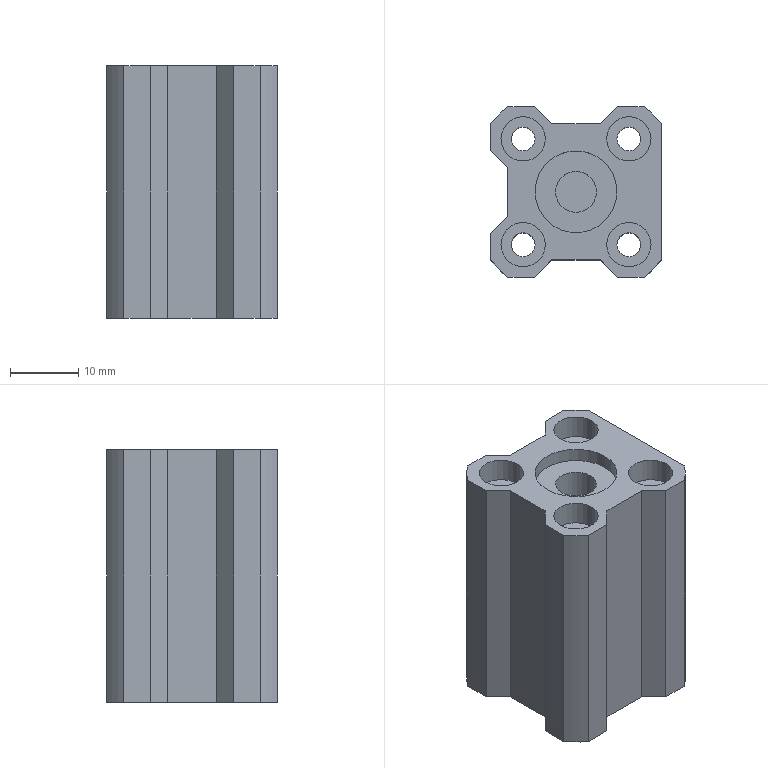Part | STEP file | 1 solid | 54 faces | box 25 x 25 x 37 mm | volume 14578 mm3 | plane 29 | cylinder 21 | cone 4 | commonest cylinder face diameters 6.5 x8 3.5 x4 32 x4 4.2 x2 12 x2 6 x1